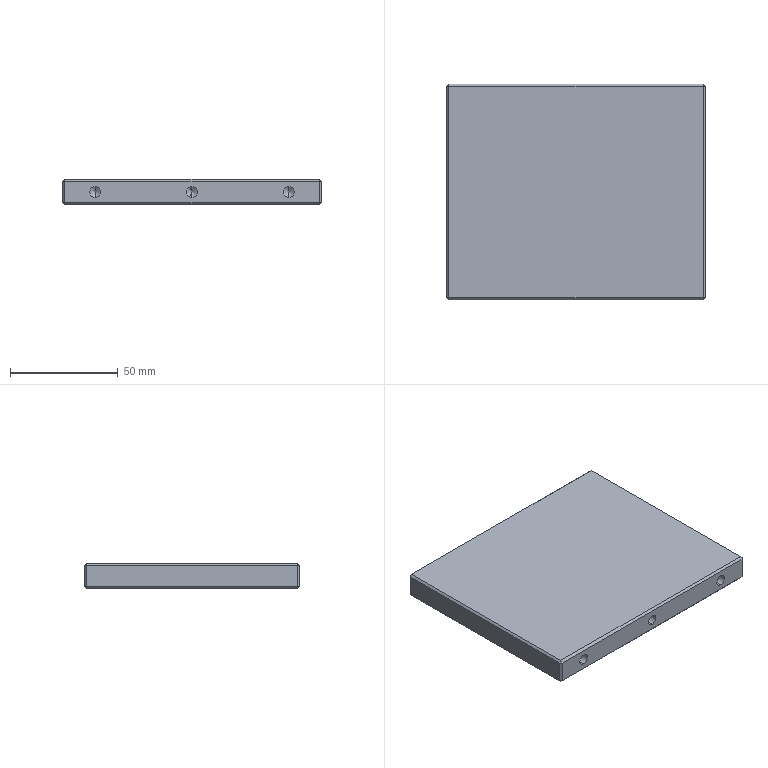Part | STEP file | 07-02 support plate | 1 solid | 49 faces | box 120 x 100 x 12 mm | volume 141828 mm3 | plane 27 | cylinder 12 | cone 10 | commonest cylinder face diameters 5 x6 4.2 x4 6 x2
STEP:
#1=CARTESIAN_POINT('',(0.,40.,3.));
#2=VERTEX_POINT('',#1);
#3=CARTESIAN_POINT('',(0.,40.,9.));
#4=VERTEX_POINT('',#3);
#5=CARTESIAN_POINT('',(0.,40.,6.));
#6=DIRECTION('',(0.,1.,0.));
#7=DIRECTION('',(0.,0.,1.));
#8=AXIS2_PLACEMENT_3D('',#5,#6,#7);
#9=CIRCLE('',#8,3.);
#10=EDGE_CURVE('',#2,#4,#9,.T.);
#11=ORIENTED_EDGE('',*,*,#10,.F.);
#12=CARTESIAN_POINT('',(0.,50.,3.));
#13=VERTEX_POINT('',#12);
#14=CARTESIAN_POINT('',(0.,40.,3.));
#15=DIRECTION('',(0.,1.,0.));
#16=VECTOR('',#15,1000.);
#17=LINE('',#14,#16);
#18=EDGE_CURVE('',#2,#13,#17,.T.);
#19=ORIENTED_EDGE('',*,*,#18,.T.);
#20=CARTESIAN_POINT('',(0.,50.,9.));
#21=VERTEX_POINT('',#20);
#22=CARTESIAN_POINT('',(0.,50.,6.));
#23=DIRECTION('',(0.,1.,0.));
#24=DIRECTION('',(0.,0.,1.));
#25=AXIS2_PLACEMENT_3D('',#22,#23,#24);
#26=CIRCLE('',#25,3.);
#27=EDGE_CURVE('',#13,#21,#26,.T.);
#28=ORIENTED_EDGE('',*,*,#27,.T.);
#29=CARTESIAN_POINT('',(0.,40.,9.));
#30=DIRECTION('',(0.,1.,0.));
#31=VECTOR('',#30,1000.);
#32=LINE('',#29,#31);
#33=EDGE_CURVE('',#4,#21,#32,.T.);
#34=ORIENTED_EDGE('',*,*,#33,.F.);
#35=EDGE_LOOP('',(#11,#19,#28,#34));
#36=FACE_OUTER_BOUND('',#35,.T.);
#37=CARTESIAN_POINT('',(0.,40.,6.));
#38=DIRECTION('',(0.,1.,0.));
#39=DIRECTION('',(0.,0.,1.));
#40=AXIS2_PLACEMENT_3D('',#37,#38,#39);
#41=CYLINDRICAL_SURFACE('',#40,3.);
#42=ADVANCED_FACE('',(#36),#41,.F.);
#43=CARTESIAN_POINT('',(-45.,36.,3.9));
#44=VERTEX_POINT('',#43);
#45=CARTESIAN_POINT('',(-45.,36.,8.1));
#46=VERTEX_POINT('',#45);
#47=CARTESIAN_POINT('',(-45.,36.,6.));
#48=DIRECTION('',(0.,1.,0.));
#49=DIRECTION('',(0.,0.,1.));
#50=AXIS2_PLACEMENT_3D('',#47,#48,#49);
#51=CIRCLE('',#50,2.1);
#52=EDGE_CURVE('',#44,#46,#51,.T.);
#53=ORIENTED_EDGE('',*,*,#52,.F.);
#54=CARTESIAN_POINT('',(-45.,50.,3.9));
#55=VERTEX_POINT('',#54);
#56=CARTESIAN_POINT('',(-45.,50.,3.9));
#57=DIRECTION('',(0.,1.,0.));
#58=VECTOR('',#57,1000.);
#59=LINE('',#56,#58);
#60=EDGE_CURVE('',#44,#55,#59,.T.);
#61=ORIENTED_EDGE('',*,*,#60,.T.);
#62=CARTESIAN_POINT('',(-45.,50.,8.1));
#63=VERTEX_POINT('',#62);
#64=CARTESIAN_POINT('',(-45.,50.,6.));
#65=DIRECTION('',(0.,1.,0.));
#66=DIRECTION('',(0.,0.,1.));
#67=AXIS2_PLACEMENT_3D('',#64,#65,#66);
#68=CIRCLE('',#67,2.1);
#69=EDGE_CURVE('',#55,#63,#68,.T.);
#70=ORIENTED_EDGE('',*,*,#69,.T.);
#71=CARTESIAN_POINT('',(-45.,50.,8.1));
#72=DIRECTION('',(0.,1.,0.));
#73=VECTOR('',#72,1000.);
#74=LINE('',#71,#73);
#75=EDGE_CURVE('',#46,#63,#74,.T.);
#76=ORIENTED_EDGE('',*,*,#75,.F.);
#77=EDGE_LOOP('',(#53,#61,#70,#76));
#78=FACE_OUTER_BOUND('',#77,.T.);
#79=CARTESIAN_POINT('',(-45.,50.,6.));
#80=DIRECTION('',(0.,1.,0.));
#81=DIRECTION('',(0.,0.,1.));
#82=AXIS2_PLACEMENT_3D('',#79,#80,#81);
#83=CYLINDRICAL_SURFACE('',#82,2.1);
#84=ADVANCED_FACE('',(#78),#83,.F.);
#85=CARTESIAN_POINT('',(-45.,34.738,6.));
#86=VERTEX_POINT('',#85);
#87=CARTESIAN_POINT('',(-45.,36.,8.1));
#88=DIRECTION('',(0.,0.515,0.8572));
#89=VECTOR('',#88,1000.);
#90=LINE('',#87,#89);
#91=EDGE_CURVE('',#86,#46,#90,.T.);
#92=ORIENTED_EDGE('',*,*,#91,.F.);
#93=CARTESIAN_POINT('',(-45.,36.,3.9));
#94=DIRECTION('',(0.,0.515,-0.8572));
#95=VECTOR('',#94,1000.);
#96=LINE('',#93,#95);
#97=EDGE_CURVE('',#86,#44,#96,.T.);
#98=ORIENTED_EDGE('',*,*,#97,.T.);
#99=ORIENTED_EDGE('',*,*,#52,.T.);
#100=EDGE_LOOP('',(#92,#98,#99));
#101=FACE_OUTER_BOUND('',#100,.T.);
#102=CARTESIAN_POINT('',(-45.,36.,6.));
#103=DIRECTION('',(0.,1.,0.));
#104=DIRECTION('',(0.,0.,1.));
#105=AXIS2_PLACEMENT_3D('',#102,#103,#104);
#106=CONICAL_SURFACE('',#105,2.1,1.03);
#107=ADVANCED_FACE('',(#101),#106,.F.);
#108=CARTESIAN_POINT('',(45.,36.,3.9));
#109=VERTEX_POINT('',#108);
#110=CARTESIAN_POINT('',(45.,36.,8.1));
#111=VERTEX_POINT('',#110);
#112=CARTESIAN_POINT('',(45.,36.,6.));
#113=DIRECTION('',(0.,1.,0.));
#114=DIRECTION('',(0.,0.,1.));
#115=AXIS2_PLACEMENT_3D('',#112,#113,#114);
#116=CIRCLE('',#115,2.1);
#117=EDGE_CURVE('',#109,#111,#116,.T.);
#118=ORIENTED_EDGE('',*,*,#117,.F.);
#119=CARTESIAN_POINT('',(45.,50.,3.9));
#120=VERTEX_POINT('',#119);
#121=CARTESIAN_POINT('',(45.,50.,3.9));
#122=DIRECTION('',(0.,1.,0.));
#123=VECTOR('',#122,1000.);
#124=LINE('',#121,#123);
#125=EDGE_CURVE('',#109,#120,#124,.T.);
#126=ORIENTED_EDGE('',*,*,#125,.T.);
#127=CARTESIAN_POINT('',(45.,50.,8.1));
#128=VERTEX_POINT('',#127);
#129=CARTESIAN_POINT('',(45.,50.,6.));
#130=DIRECTION('',(0.,1.,0.));
#131=DIRECTION('',(0.,0.,1.));
#132=AXIS2_PLACEMENT_3D('',#129,#130,#131);
#133=CIRCLE('',#132,2.1);
#134=EDGE_CURVE('',#120,#128,#133,.T.);
#135=ORIENTED_EDGE('',*,*,#134,.T.);
#136=CARTESIAN_POINT('',(45.,50.,8.1));
#137=DIRECTION('',(0.,1.,0.));
#138=VECTOR('',#137,1000.);
#139=LINE('',#136,#138);
#140=EDGE_CURVE('',#111,#128,#139,.T.);
#141=ORIENTED_EDGE('',*,*,#140,.F.);
#142=EDGE_LOOP('',(#118,#126,#135,#141));
#143=FACE_OUTER_BOUND('',#142,.T.);
#144=CARTESIAN_POINT('',(45.,50.,6.));
#145=DIRECTION('',(0.,1.,0.));
#146=DIRECTION('',(0.,0.,1.));
#147=AXIS2_PLACEMENT_3D('',#144,#145,#146);
#148=CYLINDRICAL_SURFACE('',#147,2.1);
#149=ADVANCED_FACE('',(#143),#148,.F.);
#150=CARTESIAN_POINT('',(45.,34.738,6.));
#151=VERTEX_POINT('',#150);
#152=CARTESIAN_POINT('',(45.,36.,8.1));
#153=DIRECTION('',(0.,0.515,0.8572));
#154=VECTOR('',#153,1000.);
#155=LINE('',#152,#154);
#156=EDGE_CURVE('',#151,#111,#155,.T.);
#157=ORIENTED_EDGE('',*,*,#156,.F.);
#158=CARTESIAN_POINT('',(45.,36.,3.9));
#159=DIRECTION('',(0.,0.515,-0.8572));
#160=VECTOR('',#159,1000.);
#161=LINE('',#158,#160);
#162=EDGE_CURVE('',#151,#109,#161,.T.);
#163=ORIENTED_EDGE('',*,*,#162,.T.);
#164=ORIENTED_EDGE('',*,*,#117,.T.);
#165=EDGE_LOOP('',(#157,#163,#164));
#166=FACE_OUTER_BOUND('',#165,.T.);
#167=CARTESIAN_POINT('',(45.,36.,6.));
#168=DIRECTION('',(0.,1.,0.));
#169=DIRECTION('',(0.,0.,1.));
#170=AXIS2_PLACEMENT_3D('',#167,#168,#169);
#171=CONICAL_SURFACE('',#170,2.1,1.03);
#172=ADVANCED_FACE('',(#166),#171,.F.);
#173=CARTESIAN_POINT('',(-45.,-33.,8.5));
#174=VERTEX_POINT('',#173);
#175=CARTESIAN_POINT('',(-45.,-33.,3.5));
#176=VERTEX_POINT('',#175);
#177=CARTESIAN_POINT('',(-45.,-33.,6.));
#178=DIRECTION('',(0.,-1.,0.));
#179=DIRECTION('',(0.,0.,-1.));
#180=AXIS2_PLACEMENT_3D('',#177,#178,#179);
#181=CIRCLE('',#180,2.5);
#182=EDGE_CURVE('',#174,#176,#181,.T.);
#183=ORIENTED_EDGE('',*,*,#182,.F.);
#184=CARTESIAN_POINT('',(-45.,-50.,8.5));
#185=VERTEX_POINT('',#184);
#186=CARTESIAN_POINT('',(-45.,-50.,8.5));
#187=DIRECTION('',(0.,-1.,0.));
#188=VECTOR('',#187,1000.);
#189=LINE('',#186,#188);
#190=EDGE_CURVE('',#174,#185,#189,.T.);
#191=ORIENTED_EDGE('',*,*,#190,.T.);
#192=CARTESIAN_POINT('',(-45.,-50.,3.5));
#193=VERTEX_POINT('',#192);
#194=CARTESIAN_POINT('',(-45.,-50.,6.));
#195=DIRECTION('',(0.,-1.,0.));
#196=DIRECTION('',(0.,0.,-1.));
#197=AXIS2_PLACEMENT_3D('',#194,#195,#196);
#198=CIRCLE('',#197,2.5);
#199=EDGE_CURVE('',#185,#193,#198,.T.);
#200=ORIENTED_EDGE('',*,*,#199,.T.);
#201=CARTESIAN_POINT('',(-45.,-50.,3.5));
#202=DIRECTION('',(0.,-1.,0.));
#203=VECTOR('',#202,1000.);
#204=LINE('',#201,#203);
#205=EDGE_CURVE('',#176,#193,#204,.T.);
#206=ORIENTED_EDGE('',*,*,#205,.F.);
#207=EDGE_LOOP('',(#183,#191,#200,#206));
#208=FACE_OUTER_BOUND('',#207,.T.);
#209=CARTESIAN_POINT('',(-45.,-50.,6.));
#210=DIRECTION('',(0.,-1.,0.));
#211=DIRECTION('',(0.,0.,-1.));
#212=AXIS2_PLACEMENT_3D('',#209,#210,#211);
#213=CYLINDRICAL_SURFACE('',#212,2.5);
#214=ADVANCED_FACE('',(#208),#213,.F.);
#215=CARTESIAN_POINT('',(-45.,-31.498,6.));
#216=VERTEX_POINT('',#215);
#217=CARTESIAN_POINT('',(-45.,-33.,3.5));
#218=DIRECTION('',(0.,-0.515,-0.8572));
#219=VECTOR('',#218,1000.);
#220=LINE('',#217,#219);
#221=EDGE_CURVE('',#216,#176,#220,.T.);
#222=ORIENTED_EDGE('',*,*,#221,.F.);
#223=CARTESIAN_POINT('',(-45.,-33.,8.5));
#224=DIRECTION('',(0.,-0.515,0.8572));
#225=VECTOR('',#224,1000.);
#226=LINE('',#223,#225);
#227=EDGE_CURVE('',#216,#174,#226,.T.);
#228=ORIENTED_EDGE('',*,*,#227,.T.);
#229=ORIENTED_EDGE('',*,*,#182,.T.);
#230=EDGE_LOOP('',(#222,#228,#229));
#231=FACE_OUTER_BOUND('',#230,.T.);
#232=CARTESIAN_POINT('',(-45.,-33.,6.));
#233=DIRECTION('',(0.,-1.,0.));
#234=DIRECTION('',(0.,0.,-1.));
#235=AXIS2_PLACEMENT_3D('',#232,#233,#234);
#236=CONICAL_SURFACE('',#235,2.5,1.03);
#237=ADVANCED_FACE('',(#231),#236,.F.);
#238=CARTESIAN_POINT('',(0.,-33.,8.5));
#239=VERTEX_POINT('',#238);
#240=CARTESIAN_POINT('',(0.,-33.,3.5));
#241=VERTEX_POINT('',#240);
#242=CARTESIAN_POINT('',(0.,-33.,6.));
#243=DIRECTION('',(0.,-1.,0.));
#244=DIRECTION('',(0.,0.,-1.));
#245=AXIS2_PLACEMENT_3D('',#242,#243,#244);
#246=CIRCLE('',#245,2.5);
#247=EDGE_CURVE('',#239,#241,#246,.T.);
#248=ORIENTED_EDGE('',*,*,#247,.F.);
#249=CARTESIAN_POINT('',(0.,-50.,8.5));
#250=VERTEX_POINT('',#249);
#251=CARTESIAN_POINT('',(0.,-50.,8.5));
#252=DIRECTION('',(0.,-1.,0.));
#253=VECTOR('',#252,1000.);
#254=LINE('',#251,#253);
#255=EDGE_CURVE('',#239,#250,#254,.T.);
#256=ORIENTED_EDGE('',*,*,#255,.T.);
#257=CARTESIAN_POINT('',(0.,-50.,3.5));
#258=VERTEX_POINT('',#257);
#259=CARTESIAN_POINT('',(0.,-50.,6.));
#260=DIRECTION('',(0.,-1.,0.));
#261=DIRECTION('',(0.,0.,-1.));
#262=AXIS2_PLACEMENT_3D('',#259,#260,#261);
#263=CIRCLE('',#262,2.5);
#264=EDGE_CURVE('',#250,#258,#263,.T.);
#265=ORIENTED_EDGE('',*,*,#264,.T.);
#266=CARTESIAN_POINT('',(0.,-50.,3.5));
#267=DIRECTION('',(0.,-1.,0.));
#268=VECTOR('',#267,1000.);
#269=LINE('',#266,#268);
#270=EDGE_CURVE('',#241,#258,#269,.T.);
#271=ORIENTED_EDGE('',*,*,#270,.F.);
#272=EDGE_LOOP('',(#248,#256,#265,#271));
#273=FACE_OUTER_BOUND('',#272,.T.);
#274=CARTESIAN_POINT('',(0.,-50.,6.));
#275=DIRECTION('',(0.,-1.,0.));
#276=DIRECTION('',(0.,0.,-1.));
#277=AXIS2_PLACEMENT_3D('',#274,#275,#276);
#278=CYLINDRICAL_SURFACE('',#277,2.5);
#279=ADVANCED_FACE('',(#273),#278,.F.);
#280=CARTESIAN_POINT('',(0.,-31.498,6.));
#281=VERTEX_POINT('',#280);
#282=CARTESIAN_POINT('',(0.,-33.,3.5));
#283=DIRECTION('',(0.,-0.515,-0.8572));
#284=VECTOR('',#283,1000.);
#285=LINE('',#282,#284);
#286=EDGE_CURVE('',#281,#241,#285,.T.);
#287=ORIENTED_EDGE('',*,*,#286,.F.);
#288=CARTESIAN_POINT('',(0.,-33.,8.5));
#289=DIRECTION('',(0.,-0.515,0.8572));
#290=VECTOR('',#289,1000.);
#291=LINE('',#288,#290);
#292=EDGE_CURVE('',#281,#239,#291,.T.);
#293=ORIENTED_EDGE('',*,*,#292,.T.);
#294=ORIENTED_EDGE('',*,*,#247,.T.);
#295=EDGE_LOOP('',(#287,#293,#294));
#296=FACE_OUTER_BOUND('',#295,.T.);
#297=CARTESIAN_POINT('',(0.,-33.,6.));
#298=DIRECTION('',(0.,-1.,0.));
#299=DIRECTION('',(0.,0.,-1.));
#300=AXIS2_PLACEMENT_3D('',#297,#298,#299);
#301=CONICAL_SURFACE('',#300,2.5,1.03);
#302=ADVANCED_FACE('',(#296),#301,.F.);
#303=CARTESIAN_POINT('',(45.,-33.,8.5));
#304=VERTEX_POINT('',#303);
#305=CARTESIAN_POINT('',(45.,-33.,3.5));
#306=VERTEX_POINT('',#305);
#307=CARTESIAN_POINT('',(45.,-33.,6.));
#308=DIRECTION('',(0.,-1.,0.));
#309=DIRECTION('',(0.,0.,-1.));
#310=AXIS2_PLACEMENT_3D('',#307,#308,#309);
#311=CIRCLE('',#310,2.5);
#312=EDGE_CURVE('',#304,#306,#311,.T.);
#313=ORIENTED_EDGE('',*,*,#312,.F.);
#314=CARTESIAN_POINT('',(45.,-50.,8.5));
#315=VERTEX_POINT('',#314);
#316=CARTESIAN_POINT('',(45.,-50.,8.5));
#317=DIRECTION('',(0.,-1.,0.));
#318=VECTOR('',#317,1000.);
#319=LINE('',#316,#318);
#320=EDGE_CURVE('',#304,#315,#319,.T.);
#321=ORIENTED_EDGE('',*,*,#320,.T.);
#322=CARTESIAN_POINT('',(45.,-50.,3.5));
#323=VERTEX_POINT('',#322);
#324=CARTESIAN_POINT('',(45.,-50.,6.));
#325=DIRECTION('',(0.,-1.,0.));
#326=DIRECTION('',(0.,0.,-1.));
#327=AXIS2_PLACEMENT_3D('',#324,#325,#326);
#328=CIRCLE('',#327,2.5);
#329=EDGE_CURVE('',#315,#323,#328,.T.);
#330=ORIENTED_EDGE('',*,*,#329,.T.);
#331=CARTESIAN_POINT('',(45.,-50.,3.5));
#332=DIRECTION('',(0.,-1.,0.));
#333=VECTOR('',#332,1000.);
#334=LINE('',#331,#333);
#335=EDGE_CURVE('',#306,#323,#334,.T.);
#336=ORIENTED_EDGE('',*,*,#335,.F.);
#337=EDGE_LOOP('',(#313,#321,#330,#336));
#338=FACE_OUTER_BOUND('',#337,.T.);
#339=CARTESIAN_POINT('',(45.,-50.,6.));
#340=DIRECTION('',(0.,-1.,0.));
#341=DIRECTION('',(0.,0.,-1.));
#342=AXIS2_PLACEMENT_3D('',#339,#340,#341);
#343=CYLINDRICAL_SURFACE('',#342,2.5);
#344=ADVANCED_FACE('',(#338),#343,.F.);
#345=CARTESIAN_POINT('',(45.,-31.498,6.));
#346=VERTEX_POINT('',#345);
#347=CARTESIAN_POINT('',(45.,-33.,3.5));
#348=DIRECTION('',(0.,-0.515,-0.8572));
#349=VECTOR('',#348,1000.);
#350=LINE('',#347,#349);
#351=EDGE_CURVE('',#346,#306,#350,.T.);
#352=ORIENTED_EDGE('',*,*,#351,.F.);
#353=CARTESIAN_POINT('',(45.,-33.,8.5));
#354=DIRECTION('',(0.,-0.515,0.8572));
#355=VECTOR('',#354,1000.);
#356=LINE('',#353,#355);
#357=EDGE_CURVE('',#346,#304,#356,.T.);
#358=ORIENTED_EDGE('',*,*,#357,.T.);
#359=ORIENTED_EDGE('',*,*,#312,.T.);
#360=EDGE_LOOP('',(#352,#358,#359));
#361=FACE_OUTER_BOUND('',#360,.T.);
#362=CARTESIAN_POINT('',(45.,-33.,6.));
#363=DIRECTION('',(0.,-1.,0.));
#364=DIRECTION('',(0.,0.,-1.));
#365=AXIS2_PLACEMENT_3D('',#362,#363,#364);
#366=CONICAL_SURFACE('',#365,2.5,1.03);
#367=ADVANCED_FACE('',(#361),#366,.F.);
#368=CARTESIAN_POINT('',(60.,-49.,11.));
#369=VERTEX_POINT('',#368);
#370=CARTESIAN_POINT('',(60.,-49.,1.));
#371=VERTEX_POINT('',#370);
#372=CARTESIAN_POINT('',(60.,-49.,12.));
#373=DIRECTION('',(0.,0.,-1.));
#374=VECTOR('',#373,1000.);
#375=LINE('',#372,#374);
#376=EDGE_CURVE('',#369,#371,#375,.T.);
#377=ORIENTED_EDGE('',*,*,#376,.T.);
#378=CARTESIAN_POINT('',(60.,49.,1.));
#379=VERTEX_POINT('',#378);
#380=CARTESIAN_POINT('',(60.,50.,1.));
#381=DIRECTION('',(0.,1.,0.));
#382=VECTOR('',#381,1000.);
#383=LINE('',#380,#382);
#384=EDGE_CURVE('',#371,#379,#383,.T.);
#385=ORIENTED_EDGE('',*,*,#384,.T.);
#386=CARTESIAN_POINT('',(60.,49.,11.));
#387=VERTEX_POINT('',#386);
#388=CARTESIAN_POINT('',(60.,49.,12.));
#389=DIRECTION('',(0.,0.,1.));
#390=VECTOR('',#389,1000.);
#391=LINE('',#388,#390);
#392=EDGE_CURVE('',#379,#387,#391,.T.);
#393=ORIENTED_EDGE('',*,*,#392,.T.);
#394=CARTESIAN_POINT('',(60.,-50.,11.));
#395=DIRECTION('',(0.,-1.,0.));
#396=VECTOR('',#395,1000.);
#397=LINE('',#394,#396);
#398=EDGE_CURVE('',#387,#369,#397,.T.);
#399=ORIENTED_EDGE('',*,*,#398,.T.);
#400=EDGE_LOOP('',(#377,#385,#393,#399));
#401=FACE_OUTER_BOUND('',#400,.T.);
#402=CARTESIAN_POINT('',(60.,50.,12.));
#403=DIRECTION('',(-1.,0.,0.));
#404=DIRECTION('',(0.,-1.,0.));
#405=AXIS2_PLACEMENT_3D('',#402,#403,#404);
#406=PLANE('',#405);
#407=ADVANCED_FACE('',(#401),#406,.F.);
#408=CARTESIAN_POINT('',(59.,50.,11.));
#409=VERTEX_POINT('',#408);
#410=CARTESIAN_POINT('',(59.,50.,1.));
#411=VERTEX_POINT('',#410);
#412=CARTESIAN_POINT('',(59.,50.,12.));
#413=DIRECTION('',(0.,0.,-1.));
#414=VECTOR('',#413,1000.);
#415=LINE('',#412,#414);
#416=EDGE_CURVE('',#409,#411,#415,.T.);
#417=ORIENTED_EDGE('',*,*,#416,.T.);
#418=CARTESIAN_POINT('',(-59.,50.,1.));
#419=VERTEX_POINT('',#418);
#420=CARTESIAN_POINT('',(-60.,50.,1.));
#421=DIRECTION('',(-1.,0.,0.));
#422=VECTOR('',#421,1000.);
#423=LINE('',#420,#422);
#424=EDGE_CURVE('',#411,#419,#423,.T.);
#425=ORIENTED_EDGE('',*,*,#424,.T.);
#426=CARTESIAN_POINT('',(-59.,50.,11.));
#427=VERTEX_POINT('',#426);
#428=CARTESIAN_POINT('',(-59.,50.,12.));
#429=DIRECTION('',(0.,0.,1.));
#430=VECTOR('',#429,1000.);
#431=LINE('',#428,#430);
#432=EDGE_CURVE('',#419,#427,#431,.T.);
#433=ORIENTED_EDGE('',*,*,#432,.T.);
#434=CARTESIAN_POINT('',(60.,50.,11.));
#435=DIRECTION('',(1.,0.,0.));
#436=VECTOR('',#435,1000.);
#437=LINE('',#434,#436);
#438=EDGE_CURVE('',#427,#409,#437,.T.);
#439=ORIENTED_EDGE('',*,*,#438,.T.);
#440=EDGE_LOOP('',(#417,#425,#433,#439));
#441=FACE_OUTER_BOUND('',#440,.T.);
#442=CARTESIAN_POINT('',(0.,50.,6.));
#443=DIRECTION('',(0.,1.,0.));
#444=DIRECTION('',(0.,0.,1.));
#445=AXIS2_PLACEMENT_3D('',#442,#443,#444);
#446=CIRCLE('',#445,3.);
#447=EDGE_CURVE('',#21,#13,#446,.T.);
#448=ORIENTED_EDGE('',*,*,#447,.F.);
#449=ORIENTED_EDGE('',*,*,#27,.F.);
#450=EDGE_LOOP('',(#448,#449));
#451=FACE_BOUND('',#450,.T.);
#452=CARTESIAN_POINT('',(-45.,50.,6.));
#453=DIRECTION('',(0.,1.,0.));
#454=DIRECTION('',(0.,0.,1.));
#455=AXIS2_PLACEMENT_3D('',#452,#453,#454);
#456=CIRCLE('',#455,2.1);
#457=EDGE_CURVE('',#63,#55,#456,.T.);
#458=ORIENTED_EDGE('',*,*,#457,.F.);
#459=ORIENTED_EDGE('',*,*,#69,.F.);
#460=EDGE_LOOP('',(#458,#459));
#461=FACE_BOUND('',#460,.T.);
#462=CARTESIAN_POINT('',(45.,50.,6.));
#463=DIRECTION('',(0.,1.,0.));
#464=DIRECTION('',(0.,0.,1.));
#465=AXIS2_PLACEMENT_3D('',#462,#463,#464);
#466=CIRCLE('',#465,2.1);
#467=EDGE_CURVE('',#128,#120,#466,.T.);
#468=ORIENTED_EDGE('',*,*,#467,.F.);
#469=ORIENTED_EDGE('',*,*,#134,.F.);
#470=EDGE_LOOP('',(#468,#469));
#471=FACE_BOUND('',#470,.T.);
#472=CARTESIAN_POINT('',(-60.,50.,12.));
#473=DIRECTION('',(0.,-1.,0.));
#474=DIRECTION('',(0.,0.,-1.));
#475=AXIS2_PLACEMENT_3D('',#472,#473,#474);
#476=PLANE('',#475);
#477=ADVANCED_FACE('',(#441,#451,#461,#471),#476,.F.);
#478=CARTESIAN_POINT('',(-60.,49.,11.));
#479=VERTEX_POINT('',#478);
#480=CARTESIAN_POINT('',(-60.,49.,1.));
#481=VERTEX_POINT('',#480);
#482=CARTESIAN_POINT('',(-60.,49.,12.));
#483=DIRECTION('',(0.,0.,-1.));
#484=VECTOR('',#483,1000.);
#485=LINE('',#482,#484);
#486=EDGE_CURVE('',#479,#481,#485,.T.);
#487=ORIENTED_EDGE('',*,*,#486,.T.);
#488=CARTESIAN_POINT('',(-60.,-49.,1.));
#489=VERTEX_POINT('',#488);
#490=CARTESIAN_POINT('',(-60.,50.,1.));
#491=DIRECTION('',(0.,-1.,0.));
#492=VECTOR('',#491,1000.);
#493=LINE('',#490,#492);
#494=EDGE_CURVE('',#481,#489,#493,.T.);
#495=ORIENTED_EDGE('',*,*,#494,.T.);
#496=CARTESIAN_POINT('',(-60.,-49.,11.));
#497=VERTEX_POINT('',#496);
#498=CARTESIAN_POINT('',(-60.,-49.,12.));
#499=DIRECTION('',(0.,0.,1.));
#500=VECTOR('',#499,1000.);
#501=LINE('',#498,#500);
#502=EDGE_CURVE('',#489,#497,#501,.T.);
#503=ORIENTED_EDGE('',*,*,#502,.T.);
#504=CARTESIAN_POINT('',(-60.,50.,11.));
#505=DIRECTION('',(0.,1.,0.));
#506=VECTOR('',#505,1000.);
#507=LINE('',#504,#506);
#508=EDGE_CURVE('',#497,#479,#507,.T.);
#509=ORIENTED_EDGE('',*,*,#508,.T.);
#510=EDGE_LOOP('',(#487,#495,#503,#509));
#511=FACE_OUTER_BOUND('',#510,.T.);
#512=CARTESIAN_POINT('',(-60.,50.,12.));
#513=DIRECTION('',(1.,0.,0.));
#514=DIRECTION('',(0.,1.,0.));
#515=AXIS2_PLACEMENT_3D('',#512,#513,#514);
#516=PLANE('',#515);
#517=ADVANCED_FACE('',(#511),#516,.F.);
#518=CARTESIAN_POINT('',(59.,-50.,11.));
#519=VERTEX_POINT('',#518);
#520=CARTESIAN_POINT('',(-59.,-50.,11.));
#521=VERTEX_POINT('',#520);
#522=CARTESIAN_POINT('',(-60.,-50.,11.));
#523=DIRECTION('',(-1.,0.,0.));
#524=VECTOR('',#523,1000.);
#525=LINE('',#522,#524);
#526=EDGE_CURVE('',#519,#521,#525,.T.);
#527=ORIENTED_EDGE('',*,*,#526,.T.);
#528=CARTESIAN_POINT('',(-59.,-50.,1.));
#529=VERTEX_POINT('',#528);
#530=CARTESIAN_POINT('',(-59.,-50.,12.));
#531=DIRECTION('',(0.,0.,-1.));
#532=VECTOR('',#531,1000.);
#533=LINE('',#530,#532);
#534=EDGE_CURVE('',#521,#529,#533,.T.);
#535=ORIENTED_EDGE('',*,*,#534,.T.);
#536=CARTESIAN_POINT('',(59.,-50.,1.));
#537=VERTEX_POINT('',#536);
#538=CARTESIAN_POINT('',(-60.,-50.,1.));
#539=DIRECTION('',(1.,0.,0.));
#540=VECTOR('',#539,1000.);
#541=LINE('',#538,#540);
#542=EDGE_CURVE('',#529,#537,#541,.T.);
#543=ORIENTED_EDGE('',*,*,#542,.T.);
#544=CARTESIAN_POINT('',(59.,-50.,12.));
#545=DIRECTION('',(0.,0.,1.));
#546=VECTOR('',#545,1000.);
#547=LINE('',#544,#546);
#548=EDGE_CURVE('',#537,#519,#547,.T.);
#549=ORIENTED_EDGE('',*,*,#548,.T.);
#550=EDGE_LOOP('',(#527,#535,#543,#549));
#551=FACE_OUTER_BOUND('',#550,.T.);
#552=CARTESIAN_POINT('',(-45.,-50.,6.));
#553=DIRECTION('',(0.,-1.,0.));
#554=DIRECTION('',(0.,0.,-1.));
#555=AXIS2_PLACEMENT_3D('',#552,#553,#554);
#556=CIRCLE('',#555,2.5);
#557=EDGE_CURVE('',#193,#185,#556,.T.);
#558=ORIENTED_EDGE('',*,*,#557,.F.);
#559=ORIENTED_EDGE('',*,*,#199,.F.);
#560=EDGE_LOOP('',(#558,#559));
#561=FACE_BOUND('',#560,.T.);
#562=CARTESIAN_POINT('',(0.,-50.,6.));
#563=DIRECTION('',(0.,-1.,0.));
#564=DIRECTION('',(0.,0.,-1.));
#565=AXIS2_PLACEMENT_3D('',#562,#563,#564);
#566=CIRCLE('',#565,2.5);
#567=EDGE_CURVE('',#258,#250,#566,.T.);
#568=ORIENTED_EDGE('',*,*,#567,.F.);
#569=ORIENTED_EDGE('',*,*,#264,.F.);
#570=EDGE_LOOP('',(#568,#569));
#571=FACE_BOUND('',#570,.T.);
#572=CARTESIAN_POINT('',(45.,-50.,6.));
#573=DIRECTION('',(0.,-1.,0.));
#574=DIRECTION('',(0.,0.,-1.));
#575=AXIS2_PLACEMENT_3D('',#572,#573,#574);
#576=CIRCLE('',#575,2.5);
#577=EDGE_CURVE('',#323,#315,#576,.T.);
#578=ORIENTED_EDGE('',*,*,#577,.F.);
#579=ORIENTED_EDGE('',*,*,#329,.F.);
#580=EDGE_LOOP('',(#578,#579));
#581=FACE_BOUND('',#580,.T.);
#582=CARTESIAN_POINT('',(-60.,-50.,12.));
#583=DIRECTION('',(0.,1.,0.));
#584=DIRECTION('',(0.,0.,1.));
#585=AXIS2_PLACEMENT_3D('',#582,#583,#584);
#586=PLANE('',#585);
#587=ADVANCED_FACE('',(#551,#561,#571,#581),#586,.F.);
#588=CARTESIAN_POINT('',(-59.,49.,12.));
#589=VERTEX_POINT('',#588);
#590=CARTESIAN_POINT('',(-59.,-49.,12.));
#591=VERTEX_POINT('',#590);
#592=CARTESIAN_POINT('',(-59.,-50.,12.));
#593=DIRECTION('',(0.,-1.,0.));
#594=VECTOR('',#593,1000.);
#595=LINE('',#592,#594);
#596=EDGE_CURVE('',#589,#591,#595,.T.);
#597=ORIENTED_EDGE('',*,*,#596,.T.);
#598=CARTESIAN_POINT('',(59.,-49.,12.));
#599=VERTEX_POINT('',#598);
#600=CARTESIAN_POINT('',(60.,-49.,12.));
#601=DIRECTION('',(1.,0.,0.));
#602=VECTOR('',#601,1000.);
#603=LINE('',#600,#602);
#604=EDGE_CURVE('',#591,#599,#603,.T.);
#605=ORIENTED_EDGE('',*,*,#604,.T.);
#606=CARTESIAN_POINT('',(59.,49.,12.));
#607=VERTEX_POINT('',#606);
#608=CARTESIAN_POINT('',(59.,50.,12.));
#609=DIRECTION('',(0.,1.,0.));
#610=VECTOR('',#609,1000.);
#611=LINE('',#608,#610);
#612=EDGE_CURVE('',#599,#607,#611,.T.);
#613=ORIENTED_EDGE('',*,*,#612,.T.);
#614=CARTESIAN_POINT('',(-60.,49.,12.));
#615=DIRECTION('',(-1.,0.,0.));
#616=VECTOR('',#615,1000.);
#617=LINE('',#614,#616);
#618=EDGE_CURVE('',#607,#589,#617,.T.);
#619=ORIENTED_EDGE('',*,*,#618,.T.);
#620=EDGE_LOOP('',(#597,#605,#613,#619));
#621=FACE_OUTER_BOUND('',#620,.T.);
#622=CARTESIAN_POINT('',(60.,-50.,12.));
#623=DIRECTION('',(0.,0.,1.));
#624=DIRECTION('',(1.,0.,0.));
#625=AXIS2_PLACEMENT_3D('',#622,#623,#624);
#626=PLANE('',#625);
#627=ADVANCED_FACE('',(#621),#626,.T.);
#628=CARTESIAN_POINT('',(-59.,-49.,0.));
#629=VERTEX_POINT('',#628);
#630=CARTESIAN_POINT('',(-59.,49.,0.));
#631=VERTEX_POINT('',#630);
#632=CARTESIAN_POINT('',(-59.,-50.,0.));
#633=DIRECTION('',(0.,1.,0.));
#634=VECTOR('',#633,1000.);
#635=LINE('',#632,#634);
#636=EDGE_CURVE('',#629,#631,#635,.T.);
#637=ORIENTED_EDGE('',*,*,#636,.T.);
#638=CARTESIAN_POINT('',(59.,49.,0.));
#639=VERTEX_POINT('',#638);
#640=CARTESIAN_POINT('',(60.,49.,0.));
#641=DIRECTION('',(1.,0.,0.));
#642=VECTOR('',#641,1000.);
#643=LINE('',#640,#642);
#644=EDGE_CURVE('',#631,#639,#643,.T.);
#645=ORIENTED_EDGE('',*,*,#644,.T.);
#646=CARTESIAN_POINT('',(59.,-49.,0.));
#647=VERTEX_POINT('',#646);
#648=CARTESIAN_POINT('',(59.,-50.,0.));
#649=DIRECTION('',(0.,-1.,0.));
#650=VECTOR('',#649,1000.);
#651=LINE('',#648,#650);
#652=EDGE_CURVE('',#639,#647,#651,.T.);
#653=ORIENTED_EDGE('',*,*,#652,.T.);
#654=CARTESIAN_POINT('',(60.,-49.,0.));
#655=DIRECTION('',(-1.,0.,0.));
#656=VECTOR('',#655,1000.);
#657=LINE('',#654,#656);
#658=EDGE_CURVE('',#647,#629,#657,.T.);
#659=ORIENTED_EDGE('',*,*,#658,.T.);
#660=EDGE_LOOP('',(#637,#645,#653,#659));
#661=FACE_OUTER_BOUND('',#660,.T.);
#662=CARTESIAN_POINT('',(60.,-50.,0.));
#663=DIRECTION('',(0.,0.,1.));
#664=DIRECTION('',(1.,0.,0.));
#665=AXIS2_PLACEMENT_3D('',#662,#663,#664);
#666=PLANE('',#665);
#667=ADVANCED_FACE('',(#661),#666,.F.);
#668=ORIENTED_EDGE('',*,*,#357,.F.);
#669=ORIENTED_EDGE('',*,*,#351,.T.);
#670=CARTESIAN_POINT('',(45.,-33.,6.));
#671=DIRECTION('',(0.,-1.,0.));
#672=DIRECTION('',(0.,0.,-1.));
#673=AXIS2_PLACEMENT_3D('',#670,#671,#672);
#674=CIRCLE('',#673,2.5);
#675=EDGE_CURVE('',#306,#304,#674,.T.);
#676=ORIENTED_EDGE('',*,*,#675,.T.);
#677=EDGE_LOOP('',(#668,#669,#676));
#678=FACE_OUTER_BOUND('',#677,.T.);
#679=CARTESIAN_POINT('',(45.,-33.,6.));
#680=DIRECTION('',(0.,-1.,0.));
#681=DIRECTION('',(0.,0.,-1.));
#682=AXIS2_PLACEMENT_3D('',#679,#680,#681);
#683=CONICAL_SURFACE('',#682,2.5,1.03);
#684=ADVANCED_FACE('',(#678),#683,.F.);
#685=ORIENTED_EDGE('',*,*,#320,.F.);
#686=ORIENTED_EDGE('',*,*,#675,.F.);
#687=ORIENTED_EDGE('',*,*,#335,.T.);
#688=ORIENTED_EDGE('',*,*,#577,.T.);
#689=EDGE_LOOP('',(#685,#686,#687,#688));
#690=FACE_OUTER_BOUND('',#689,.T.);
#691=CARTESIAN_POINT('',(45.,-50.,6.));
#692=DIRECTION('',(0.,-1.,0.));
#693=DIRECTION('',(0.,0.,-1.));
#694=AXIS2_PLACEMENT_3D('',#691,#692,#693);
#695=CYLINDRICAL_SURFACE('',#694,2.5);
#696=ADVANCED_FACE('',(#690),#695,.F.);
#697=ORIENTED_EDGE('',*,*,#292,.F.);
#698=ORIENTED_EDGE('',*,*,#286,.T.);
#699=CARTESIAN_POINT('',(0.,-33.,6.));
#700=DIRECTION('',(0.,-1.,0.));
#701=DIRECTION('',(0.,0.,-1.));
#702=AXIS2_PLACEMENT_3D('',#699,#700,#701);
#703=CIRCLE('',#702,2.5);
#704=EDGE_CURVE('',#241,#239,#703,.T.);
#705=ORIENTED_EDGE('',*,*,#704,.T.);
#706=EDGE_LOOP('',(#697,#698,#705));
#707=FACE_OUTER_BOUND('',#706,.T.);
#708=CARTESIAN_POINT('',(0.,-33.,6.));
#709=DIRECTION('',(0.,-1.,0.));
#710=DIRECTION('',(0.,0.,-1.));
#711=AXIS2_PLACEMENT_3D('',#708,#709,#710);
#712=CONICAL_SURFACE('',#711,2.5,1.03);
#713=ADVANCED_FACE('',(#707),#712,.F.);
#714=ORIENTED_EDGE('',*,*,#255,.F.);
#715=ORIENTED_EDGE('',*,*,#704,.F.);
#716=ORIENTED_EDGE('',*,*,#270,.T.);
#717=ORIENTED_EDGE('',*,*,#567,.T.);
#718=EDGE_LOOP('',(#714,#715,#716,#717));
#719=FACE_OUTER_BOUND('',#718,.T.);
#720=CARTESIAN_POINT('',(0.,-50.,6.));
#721=DIRECTION('',(0.,-1.,0.));
#722=DIRECTION('',(0.,0.,-1.));
#723=AXIS2_PLACEMENT_3D('',#720,#721,#722);
#724=CYLINDRICAL_SURFACE('',#723,2.5);
#725=ADVANCED_FACE('',(#719),#724,.F.);
#726=ORIENTED_EDGE('',*,*,#227,.F.);
#727=ORIENTED_EDGE('',*,*,#221,.T.);
#728=CARTESIAN_POINT('',(-45.,-33.,6.));
#729=DIRECTION('',(0.,-1.,0.));
#730=DIRECTION('',(0.,0.,-1.));
#731=AXIS2_PLACEMENT_3D('',#728,#729,#730);
#732=CIRCLE('',#731,2.5);
#733=EDGE_CURVE('',#176,#174,#732,.T.);
#734=ORIENTED_EDGE('',*,*,#733,.T.);
#735=EDGE_LOOP('',(#726,#727,#734));
#736=FACE_OUTER_BOUND('',#735,.T.);
#737=CARTESIAN_POINT('',(-45.,-33.,6.));
#738=DIRECTION('',(0.,-1.,0.));
#739=DIRECTION('',(0.,0.,-1.));
#740=AXIS2_PLACEMENT_3D('',#737,#738,#739);
#741=CONICAL_SURFACE('',#740,2.5,1.03);
#742=ADVANCED_FACE('',(#736),#741,.F.);
#743=ORIENTED_EDGE('',*,*,#190,.F.);
#744=ORIENTED_EDGE('',*,*,#733,.F.);
#745=ORIENTED_EDGE('',*,*,#205,.T.);
#746=ORIENTED_EDGE('',*,*,#557,.T.);
#747=EDGE_LOOP('',(#743,#744,#745,#746));
#748=FACE_OUTER_BOUND('',#747,.T.);
#749=CARTESIAN_POINT('',(-45.,-50.,6.));
#750=DIRECTION('',(0.,-1.,0.));
#751=DIRECTION('',(0.,0.,-1.));
#752=AXIS2_PLACEMENT_3D('',#749,#750,#751);
#753=CYLINDRICAL_SURFACE('',#752,2.5);
#754=ADVANCED_FACE('',(#748),#753,.F.);
#755=ORIENTED_EDGE('',*,*,#162,.F.);
#756=ORIENTED_EDGE('',*,*,#156,.T.);
#757=CARTESIAN_POINT('',(45.,36.,6.));
#758=DIRECTION('',(0.,1.,0.));
#759=DIRECTION('',(0.,0.,1.));
#760=AXIS2_PLACEMENT_3D('',#757,#758,#759);
#761=CIRCLE('',#760,2.1);
#762=EDGE_CURVE('',#111,#109,#761,.T.);
#763=ORIENTED_EDGE('',*,*,#762,.T.);
#764=EDGE_LOOP('',(#755,#756,#763));
#765=FACE_OUTER_BOUND('',#764,.T.);
#766=CARTESIAN_POINT('',(45.,36.,6.));
#767=DIRECTION('',(0.,1.,0.));
#768=DIRECTION('',(0.,0.,1.));
#769=AXIS2_PLACEMENT_3D('',#766,#767,#768);
#770=CONICAL_SURFACE('',#769,2.1,1.03);
#771=ADVANCED_FACE('',(#765),#770,.F.);
#772=ORIENTED_EDGE('',*,*,#125,.F.);
#773=ORIENTED_EDGE('',*,*,#762,.F.);
#774=ORIENTED_EDGE('',*,*,#140,.T.);
#775=ORIENTED_EDGE('',*,*,#467,.T.);
#776=EDGE_LOOP('',(#772,#773,#774,#775));
#777=FACE_OUTER_BOUND('',#776,.T.);
#778=CARTESIAN_POINT('',(45.,50.,6.));
#779=DIRECTION('',(0.,1.,0.));
#780=DIRECTION('',(0.,0.,1.));
#781=AXIS2_PLACEMENT_3D('',#778,#779,#780);
#782=CYLINDRICAL_SURFACE('',#781,2.1);
#783=ADVANCED_FACE('',(#777),#782,.F.);
#784=ORIENTED_EDGE('',*,*,#97,.F.);
#785=ORIENTED_EDGE('',*,*,#91,.T.);
#786=CARTESIAN_POINT('',(-45.,36.,6.));
#787=DIRECTION('',(0.,1.,0.));
#788=DIRECTION('',(0.,0.,1.));
#789=AXIS2_PLACEMENT_3D('',#786,#787,#788);
#790=CIRCLE('',#789,2.1);
#791=EDGE_CURVE('',#46,#44,#790,.T.);
#792=ORIENTED_EDGE('',*,*,#791,.T.);
#793=EDGE_LOOP('',(#784,#785,#792));
#794=FACE_OUTER_BOUND('',#793,.T.);
#795=CARTESIAN_POINT('',(-45.,36.,6.));
#796=DIRECTION('',(0.,1.,0.));
#797=DIRECTION('',(0.,0.,1.));
#798=AXIS2_PLACEMENT_3D('',#795,#796,#797);
#799=CONICAL_SURFACE('',#798,2.1,1.03);
#800=ADVANCED_FACE('',(#794),#799,.F.);
#801=ORIENTED_EDGE('',*,*,#60,.F.);
#802=ORIENTED_EDGE('',*,*,#791,.F.);
#803=ORIENTED_EDGE('',*,*,#75,.T.);
#804=ORIENTED_EDGE('',*,*,#457,.T.);
#805=EDGE_LOOP('',(#801,#802,#803,#804));
#806=FACE_OUTER_BOUND('',#805,.T.);
#807=CARTESIAN_POINT('',(-45.,50.,6.));
#808=DIRECTION('',(0.,1.,0.));
#809=DIRECTION('',(0.,0.,1.));
#810=AXIS2_PLACEMENT_3D('',#807,#808,#809);
#811=CYLINDRICAL_SURFACE('',#810,2.1);
#812=ADVANCED_FACE('',(#806),#811,.F.);
#813=ORIENTED_EDGE('',*,*,#18,.F.);
#814=CARTESIAN_POINT('',(0.,40.,6.));
#815=DIRECTION('',(0.,1.,0.));
#816=DIRECTION('',(0.,0.,1.));
#817=AXIS2_PLACEMENT_3D('',#814,#815,#816);
#818=CIRCLE('',#817,3.);
#819=EDGE_CURVE('',#4,#2,#818,.T.);
#820=ORIENTED_EDGE('',*,*,#819,.F.);
#821=ORIENTED_EDGE('',*,*,#33,.T.);
#822=ORIENTED_EDGE('',*,*,#447,.T.);
#823=EDGE_LOOP('',(#813,#820,#821,#822));
#824=FACE_OUTER_BOUND('',#823,.T.);
#825=CARTESIAN_POINT('',(0.,40.,6.));
#826=DIRECTION('',(0.,1.,0.));
#827=DIRECTION('',(0.,0.,1.));
#828=AXIS2_PLACEMENT_3D('',#825,#826,#827);
#829=CYLINDRICAL_SURFACE('',#828,3.);
#830=ADVANCED_FACE('',(#824),#829,.F.);
#831=ORIENTED_EDGE('',*,*,#819,.T.);
#832=ORIENTED_EDGE('',*,*,#10,.T.);
#833=EDGE_LOOP('',(#831,#832));
#834=FACE_OUTER_BOUND('',#833,.T.);
#835=CARTESIAN_POINT('',(0.,40.,6.));
#836=DIRECTION('',(0.,1.,0.));
#837=DIRECTION('',(0.,0.,1.));
#838=AXIS2_PLACEMENT_3D('',#835,#836,#837);
#839=PLANE('',#838);
#840=ADVANCED_FACE('',(#834),#839,.T.);
#841=CARTESIAN_POINT('',(59.,-49.,12.));
#842=DIRECTION('',(0.,-0.7071,-0.7071));
#843=VECTOR('',#842,1000.);
#844=LINE('',#841,#843);
#845=EDGE_CURVE('',#599,#519,#844,.T.);
#846=ORIENTED_EDGE('',*,*,#845,.F.);
#847=ORIENTED_EDGE('',*,*,#604,.F.);
#848=CARTESIAN_POINT('',(-59.,-50.,11.));
#849=DIRECTION('',(0.,0.7071,0.7071));
#850=VECTOR('',#849,1000.);
#851=LINE('',#848,#850);
#852=EDGE_CURVE('',#521,#591,#851,.T.);
#853=ORIENTED_EDGE('',*,*,#852,.F.);
#854=ORIENTED_EDGE('',*,*,#526,.F.);
#855=EDGE_LOOP('',(#846,#847,#853,#854));
#856=FACE_OUTER_BOUND('',#855,.T.);
#857=CARTESIAN_POINT('',(60.,-49.,12.));
#858=DIRECTION('',(0.,-0.7071,0.7071));
#859=DIRECTION('',(0.,-0.7071,-0.7071));
#860=AXIS2_PLACEMENT_3D('',#857,#858,#859);
#861=PLANE('',#860);
#862=ADVANCED_FACE('',(#856),#861,.T.);
#863=CARTESIAN_POINT('',(59.,-49.,12.));
#864=DIRECTION('',(0.7071,0.,-0.7071));
#865=VECTOR('',#864,1000.);
#866=LINE('',#863,#865);
#867=EDGE_CURVE('',#599,#369,#866,.T.);
#868=ORIENTED_EDGE('',*,*,#867,.F.);
#869=ORIENTED_EDGE('',*,*,#845,.T.);
#870=CARTESIAN_POINT('',(59.5,-49.5,11.));
#871=DIRECTION('',(-0.7071,-0.7071,0.));
#872=VECTOR('',#871,1000.);
#873=LINE('',#870,#872);
#874=EDGE_CURVE('',#369,#519,#873,.T.);
#875=ORIENTED_EDGE('',*,*,#874,.F.);
#876=EDGE_LOOP('',(#868,#869,#875));
#877=FACE_OUTER_BOUND('',#876,.T.);
#878=CARTESIAN_POINT('',(59.,-49.,12.));
#879=DIRECTION('',(0.5774,-0.5774,0.5774));
#880=DIRECTION('',(0.7071,0.7071,0.));
#881=AXIS2_PLACEMENT_3D('',#878,#879,#880);
#882=PLANE('',#881);
#883=ADVANCED_FACE('',(#877),#882,.T.);
#884=CARTESIAN_POINT('',(-59.,-50.,11.));
#885=DIRECTION('',(-0.7071,0.7071,0.));
#886=VECTOR('',#885,1000.);
#887=LINE('',#884,#886);
#888=EDGE_CURVE('',#521,#497,#887,.T.);
#889=ORIENTED_EDGE('',*,*,#888,.F.);
#890=ORIENTED_EDGE('',*,*,#852,.T.);
#891=CARTESIAN_POINT('',(-59.5,-49.,11.5));
#892=DIRECTION('',(0.7071,0.,0.7071));
#893=VECTOR('',#892,1000.);
#894=LINE('',#891,#893);
#895=EDGE_CURVE('',#497,#591,#894,.T.);
#896=ORIENTED_EDGE('',*,*,#895,.F.);
#897=EDGE_LOOP('',(#889,#890,#896));
#898=FACE_OUTER_BOUND('',#897,.T.);
#899=CARTESIAN_POINT('',(-59.,-50.,11.));
#900=DIRECTION('',(-0.5774,-0.5774,0.5774));
#901=DIRECTION('',(0.,-0.7071,-0.7071));
#902=AXIS2_PLACEMENT_3D('',#899,#900,#901);
#903=PLANE('',#902);
#904=ADVANCED_FACE('',(#898),#903,.T.);
#905=ORIENTED_EDGE('',*,*,#874,.T.);
#906=ORIENTED_EDGE('',*,*,#548,.F.);
#907=CARTESIAN_POINT('',(59.,-50.,1.));
#908=DIRECTION('',(-0.7071,-0.7071,0.));
#909=VECTOR('',#908,1000.);
#910=LINE('',#907,#909);
#911=EDGE_CURVE('',#371,#537,#910,.T.);
#912=ORIENTED_EDGE('',*,*,#911,.F.);
#913=ORIENTED_EDGE('',*,*,#376,.F.);
#914=EDGE_LOOP('',(#905,#906,#912,#913));
#915=FACE_OUTER_BOUND('',#914,.T.);
#916=CARTESIAN_POINT('',(60.,-49.,12.));
#917=DIRECTION('',(-0.7071,0.7071,0.));
#918=DIRECTION('',(-0.7071,-0.7071,0.));
#919=AXIS2_PLACEMENT_3D('',#916,#917,#918);
#920=PLANE('',#919);
#921=ADVANCED_FACE('',(#915),#920,.F.);
#922=ORIENTED_EDGE('',*,*,#867,.T.);
#923=ORIENTED_EDGE('',*,*,#398,.F.);
#924=CARTESIAN_POINT('',(59.,49.,12.));
#925=DIRECTION('',(0.7071,0.,-0.7071));
#926=VECTOR('',#925,1000.);
#927=LINE('',#924,#926);
#928=EDGE_CURVE('',#607,#387,#927,.T.);
#929=ORIENTED_EDGE('',*,*,#928,.F.);
#930=ORIENTED_EDGE('',*,*,#612,.F.);
#931=EDGE_LOOP('',(#922,#923,#929,#930));
#932=FACE_OUTER_BOUND('',#931,.T.);
#933=CARTESIAN_POINT('',(59.,-50.,12.));
#934=DIRECTION('',(0.7071,0.,0.7071));
#935=DIRECTION('',(0.7071,0.,-0.7071));
#936=AXIS2_PLACEMENT_3D('',#933,#934,#935);
#937=PLANE('',#936);
#938=ADVANCED_FACE('',(#932),#937,.T.);
#939=CARTESIAN_POINT('',(-59.,49.5,11.5));
#940=DIRECTION('',(0.,0.7071,-0.7071));
#941=VECTOR('',#940,1000.);
#942=LINE('',#939,#941);
#943=EDGE_CURVE('',#589,#427,#942,.T.);
#944=ORIENTED_EDGE('',*,*,#943,.F.);
#945=ORIENTED_EDGE('',*,*,#618,.F.);
#946=CARTESIAN_POINT('',(59.,49.,12.));
#947=DIRECTION('',(0.,-0.7071,0.7071));
#948=VECTOR('',#947,1000.);
#949=LINE('',#946,#948);
#950=EDGE_CURVE('',#409,#607,#949,.T.);
#951=ORIENTED_EDGE('',*,*,#950,.F.);
#952=ORIENTED_EDGE('',*,*,#438,.F.);
#953=EDGE_LOOP('',(#944,#945,#951,#952));
#954=FACE_OUTER_BOUND('',#953,.T.);
#955=CARTESIAN_POINT('',(60.,49.,12.));
#956=DIRECTION('',(0.,0.7071,0.7071));
#957=DIRECTION('',(0.,-0.7071,0.7071));
#958=AXIS2_PLACEMENT_3D('',#955,#956,#957);
#959=PLANE('',#958);
#960=ADVANCED_FACE('',(#954),#959,.T.);
#961=ORIENTED_EDGE('',*,*,#895,.T.);
#962=ORIENTED_EDGE('',*,*,#596,.F.);
#963=CARTESIAN_POINT('',(-60.,49.,11.));
#964=DIRECTION('',(0.7071,0.,0.7071));
#965=VECTOR('',#964,1000.);
#966=LINE('',#963,#965);
#967=EDGE_CURVE('',#479,#589,#966,.T.);
#968=ORIENTED_EDGE('',*,*,#967,.F.);
#969=ORIENTED_EDGE('',*,*,#508,.F.);
#970=EDGE_LOOP('',(#961,#962,#968,#969));
#971=FACE_OUTER_BOUND('',#970,.T.);
#972=CARTESIAN_POINT('',(-59.,-50.,12.));
#973=DIRECTION('',(-0.7071,0.,0.7071));
#974=DIRECTION('',(0.7071,0.,0.7071));
#975=AXIS2_PLACEMENT_3D('',#972,#973,#974);
#976=PLANE('',#975);
#977=ADVANCED_FACE('',(#971),#976,.T.);
#978=ORIENTED_EDGE('',*,*,#888,.T.);
#979=ORIENTED_EDGE('',*,*,#502,.F.);
#980=CARTESIAN_POINT('',(-60.,-49.,1.));
#981=DIRECTION('',(-0.7071,0.7071,0.));
#982=VECTOR('',#981,1000.);
#983=LINE('',#980,#982);
#984=EDGE_CURVE('',#529,#489,#983,.T.);
#985=ORIENTED_EDGE('',*,*,#984,.F.);
#986=ORIENTED_EDGE('',*,*,#534,.F.);
#987=EDGE_LOOP('',(#978,#979,#985,#986));
#988=FACE_OUTER_BOUND('',#987,.T.);
#989=CARTESIAN_POINT('',(-59.,-50.,12.));
#990=DIRECTION('',(0.7071,0.7071,0.));
#991=DIRECTION('',(-0.7071,0.7071,0.));
#992=AXIS2_PLACEMENT_3D('',#989,#990,#991);
#993=PLANE('',#992);
#994=ADVANCED_FACE('',(#988),#993,.F.);
#995=CARTESIAN_POINT('',(59.,-50.,1.));
#996=DIRECTION('',(0.,0.7071,-0.7071));
#997=VECTOR('',#996,1000.);
#998=LINE('',#995,#997);
#999=EDGE_CURVE('',#537,#647,#998,.T.);
#1000=ORIENTED_EDGE('',*,*,#999,.F.);
#1001=ORIENTED_EDGE('',*,*,#542,.F.);
#1002=CARTESIAN_POINT('',(-59.,-49.5,0.5));
#1003=DIRECTION('',(0.,-0.7071,0.7071));
#1004=VECTOR('',#1003,1000.);
#1005=LINE('',#1002,#1004);
#1006=EDGE_CURVE('',#629,#529,#1005,.T.);
#1007=ORIENTED_EDGE('',*,*,#1006,.F.);
#1008=ORIENTED_EDGE('',*,*,#658,.F.);
#1009=EDGE_LOOP('',(#1000,#1001,#1007,#1008));
#1010=FACE_OUTER_BOUND('',#1009,.T.);
#1011=CARTESIAN_POINT('',(-60.,-50.,1.));
#1012=DIRECTION('',(0.,0.7071,0.7071));
#1013=DIRECTION('',(0.,-0.7071,0.7071));
#1014=AXIS2_PLACEMENT_3D('',#1011,#1012,#1013);
#1015=PLANE('',#1014);
#1016=ADVANCED_FACE('',(#1010),#1015,.F.);
#1017=ORIENTED_EDGE('',*,*,#911,.T.);
#1018=ORIENTED_EDGE('',*,*,#999,.T.);
#1019=CARTESIAN_POINT('',(59.5,-49.,0.5));
#1020=DIRECTION('',(-0.7071,0.,-0.7071));
#1021=VECTOR('',#1020,1000.);
#1022=LINE('',#1019,#1021);
#1023=EDGE_CURVE('',#371,#647,#1022,.T.);
#1024=ORIENTED_EDGE('',*,*,#1023,.F.);
#1025=EDGE_LOOP('',(#1017,#1018,#1024));
#1026=FACE_OUTER_BOUND('',#1025,.T.);
#1027=CARTESIAN_POINT('',(59.,-50.,1.));
#1028=DIRECTION('',(0.5774,-0.5774,-0.5774));
#1029=DIRECTION('',(0.,0.7071,-0.7071));
#1030=AXIS2_PLACEMENT_3D('',#1027,#1028,#1029);
#1031=PLANE('',#1030);
#1032=ADVANCED_FACE('',(#1026),#1031,.T.);
#1033=ORIENTED_EDGE('',*,*,#950,.T.);
#1034=ORIENTED_EDGE('',*,*,#928,.T.);
#1035=CARTESIAN_POINT('',(59.5,49.5,11.));
#1036=DIRECTION('',(0.7071,-0.7071,0.));
#1037=VECTOR('',#1036,1000.);
#1038=LINE('',#1035,#1037);
#1039=EDGE_CURVE('',#409,#387,#1038,.T.);
#1040=ORIENTED_EDGE('',*,*,#1039,.F.);
#1041=EDGE_LOOP('',(#1033,#1034,#1040));
#1042=FACE_OUTER_BOUND('',#1041,.T.);
#1043=CARTESIAN_POINT('',(59.,49.,12.));
#1044=DIRECTION('',(0.5774,0.5774,0.5774));
#1045=DIRECTION('',(-0.7071,0.7071,0.));
#1046=AXIS2_PLACEMENT_3D('',#1043,#1044,#1045);
#1047=PLANE('',#1046);
#1048=ADVANCED_FACE('',(#1042),#1047,.T.);
#1049=ORIENTED_EDGE('',*,*,#967,.T.);
#1050=ORIENTED_EDGE('',*,*,#943,.T.);
#1051=CARTESIAN_POINT('',(-60.,49.,11.));
#1052=DIRECTION('',(0.7071,0.7071,0.));
#1053=VECTOR('',#1052,1000.);
#1054=LINE('',#1051,#1053);
#1055=EDGE_CURVE('',#479,#427,#1054,.T.);
#1056=ORIENTED_EDGE('',*,*,#1055,.F.);
#1057=EDGE_LOOP('',(#1049,#1050,#1056));
#1058=FACE_OUTER_BOUND('',#1057,.T.);
#1059=CARTESIAN_POINT('',(-60.,49.,11.));
#1060=DIRECTION('',(-0.5774,0.5774,0.5774));
#1061=DIRECTION('',(0.,-0.7071,0.7071));
#1062=AXIS2_PLACEMENT_3D('',#1059,#1060,#1061);
#1063=PLANE('',#1062);
#1064=ADVANCED_FACE('',(#1058),#1063,.T.);
#1065=ORIENTED_EDGE('',*,*,#1006,.T.);
#1066=ORIENTED_EDGE('',*,*,#984,.T.);
#1067=CARTESIAN_POINT('',(-60.,-49.,1.));
#1068=DIRECTION('',(-0.7071,0.,0.7071));
#1069=VECTOR('',#1068,1000.);
#1070=LINE('',#1067,#1069);
#1071=EDGE_CURVE('',#629,#489,#1070,.T.);
#1072=ORIENTED_EDGE('',*,*,#1071,.F.);
#1073=EDGE_LOOP('',(#1065,#1066,#1072));
#1074=FACE_OUTER_BOUND('',#1073,.T.);
#1075=CARTESIAN_POINT('',(-60.,-49.,1.));
#1076=DIRECTION('',(-0.5774,-0.5774,-0.5774));
#1077=DIRECTION('',(0.,0.7071,-0.7071));
#1078=AXIS2_PLACEMENT_3D('',#1075,#1076,#1077);
#1079=PLANE('',#1078);
#1080=ADVANCED_FACE('',(#1074),#1079,.T.);
#1081=ORIENTED_EDGE('',*,*,#1023,.T.);
#1082=ORIENTED_EDGE('',*,*,#652,.F.);
#1083=CARTESIAN_POINT('',(59.,49.,0.));
#1084=DIRECTION('',(-0.7071,0.,-0.7071));
#1085=VECTOR('',#1084,1000.);
#1086=LINE('',#1083,#1085);
#1087=EDGE_CURVE('',#379,#639,#1086,.T.);
#1088=ORIENTED_EDGE('',*,*,#1087,.F.);
#1089=ORIENTED_EDGE('',*,*,#384,.F.);
#1090=EDGE_LOOP('',(#1081,#1082,#1088,#1089));
#1091=FACE_OUTER_BOUND('',#1090,.T.);
#1092=CARTESIAN_POINT('',(60.,50.,1.));
#1093=DIRECTION('',(-0.7071,0.,0.7071));
#1094=DIRECTION('',(0.7071,0.,0.7071));
#1095=AXIS2_PLACEMENT_3D('',#1092,#1093,#1094);
#1096=PLANE('',#1095);
#1097=ADVANCED_FACE('',(#1091),#1096,.F.);
#1098=ORIENTED_EDGE('',*,*,#1039,.T.);
#1099=ORIENTED_EDGE('',*,*,#392,.F.);
#1100=CARTESIAN_POINT('',(59.5,49.5,1.));
#1101=DIRECTION('',(0.7071,-0.7071,0.));
#1102=VECTOR('',#1101,1000.);
#1103=LINE('',#1100,#1102);
#1104=EDGE_CURVE('',#411,#379,#1103,.T.);
#1105=ORIENTED_EDGE('',*,*,#1104,.F.);
#1106=ORIENTED_EDGE('',*,*,#416,.F.);
#1107=EDGE_LOOP('',(#1098,#1099,#1105,#1106));
#1108=FACE_OUTER_BOUND('',#1107,.T.);
#1109=CARTESIAN_POINT('',(59.,50.,12.));
#1110=DIRECTION('',(-0.7071,-0.7071,0.));
#1111=DIRECTION('',(0.7071,-0.7071,0.));
#1112=AXIS2_PLACEMENT_3D('',#1109,#1110,#1111);
#1113=PLANE('',#1112);
#1114=ADVANCED_FACE('',(#1108),#1113,.F.);
#1115=ORIENTED_EDGE('',*,*,#1055,.T.);
#1116=ORIENTED_EDGE('',*,*,#432,.F.);
#1117=CARTESIAN_POINT('',(-59.,50.,1.));
#1118=DIRECTION('',(0.7071,0.7071,0.));
#1119=VECTOR('',#1118,1000.);
#1120=LINE('',#1117,#1119);
#1121=EDGE_CURVE('',#481,#419,#1120,.T.);
#1122=ORIENTED_EDGE('',*,*,#1121,.F.);
#1123=ORIENTED_EDGE('',*,*,#486,.F.);
#1124=EDGE_LOOP('',(#1115,#1116,#1122,#1123));
#1125=FACE_OUTER_BOUND('',#1124,.T.);
#1126=CARTESIAN_POINT('',(-60.,49.,12.));
#1127=DIRECTION('',(0.7071,-0.7071,0.));
#1128=DIRECTION('',(0.7071,0.7071,0.));
#1129=AXIS2_PLACEMENT_3D('',#1126,#1127,#1128);
#1130=PLANE('',#1129);
#1131=ADVANCED_FACE('',(#1125),#1130,.F.);
#1132=ORIENTED_EDGE('',*,*,#1071,.T.);
#1133=ORIENTED_EDGE('',*,*,#494,.F.);
#1134=CARTESIAN_POINT('',(-59.5,49.,0.5));
#1135=DIRECTION('',(-0.7071,0.,0.7071));
#1136=VECTOR('',#1135,1000.);
#1137=LINE('',#1134,#1136);
#1138=EDGE_CURVE('',#631,#481,#1137,.T.);
#1139=ORIENTED_EDGE('',*,*,#1138,.F.);
#1140=ORIENTED_EDGE('',*,*,#636,.F.);
#1141=EDGE_LOOP('',(#1132,#1133,#1139,#1140));
#1142=FACE_OUTER_BOUND('',#1141,.T.);
#1143=CARTESIAN_POINT('',(-60.,50.,1.));
#1144=DIRECTION('',(0.7071,0.,0.7071));
#1145=DIRECTION('',(0.7071,0.,-0.7071));
#1146=AXIS2_PLACEMENT_3D('',#1143,#1144,#1145);
#1147=PLANE('',#1146);
#1148=ADVANCED_FACE('',(#1142),#1147,.F.);
#1149=ORIENTED_EDGE('',*,*,#1104,.T.);
#1150=ORIENTED_EDGE('',*,*,#1087,.T.);
#1151=CARTESIAN_POINT('',(59.,49.,0.));
#1152=DIRECTION('',(0.,-0.7071,-0.7071));
#1153=VECTOR('',#1152,1000.);
#1154=LINE('',#1151,#1153);
#1155=EDGE_CURVE('',#411,#639,#1154,.T.);
#1156=ORIENTED_EDGE('',*,*,#1155,.F.);
#1157=EDGE_LOOP('',(#1149,#1150,#1156));
#1158=FACE_OUTER_BOUND('',#1157,.T.);
#1159=CARTESIAN_POINT('',(59.,49.,0.));
#1160=DIRECTION('',(0.5774,0.5774,-0.5774));
#1161=DIRECTION('',(0.,0.7071,0.7071));
#1162=AXIS2_PLACEMENT_3D('',#1159,#1160,#1161);
#1163=PLANE('',#1162);
#1164=ADVANCED_FACE('',(#1158),#1163,.T.);
#1165=ORIENTED_EDGE('',*,*,#1138,.T.);
#1166=ORIENTED_EDGE('',*,*,#1121,.T.);
#1167=CARTESIAN_POINT('',(-59.,50.,1.));
#1168=DIRECTION('',(0.,0.7071,0.7071));
#1169=VECTOR('',#1168,1000.);
#1170=LINE('',#1167,#1169);
#1171=EDGE_CURVE('',#631,#419,#1170,.T.);
#1172=ORIENTED_EDGE('',*,*,#1171,.F.);
#1173=EDGE_LOOP('',(#1165,#1166,#1172));
#1174=FACE_OUTER_BOUND('',#1173,.T.);
#1175=CARTESIAN_POINT('',(-59.,50.,1.));
#1176=DIRECTION('',(-0.5774,0.5774,-0.5774));
#1177=DIRECTION('',(0.,0.7071,0.7071));
#1178=AXIS2_PLACEMENT_3D('',#1175,#1176,#1177);
#1179=PLANE('',#1178);
#1180=ADVANCED_FACE('',(#1174),#1179,.T.);
#1181=ORIENTED_EDGE('',*,*,#1155,.T.);
#1182=ORIENTED_EDGE('',*,*,#644,.F.);
#1183=ORIENTED_EDGE('',*,*,#1171,.T.);
#1184=ORIENTED_EDGE('',*,*,#424,.F.);
#1185=EDGE_LOOP('',(#1181,#1182,#1183,#1184));
#1186=FACE_OUTER_BOUND('',#1185,.T.);
#1187=CARTESIAN_POINT('',(-60.,50.,1.));
#1188=DIRECTION('',(0.,-0.7071,0.7071));
#1189=DIRECTION('',(0.,-0.7071,-0.7071));
#1190=AXIS2_PLACEMENT_3D('',#1187,#1188,#1189);
#1191=PLANE('',#1190);
#1192=ADVANCED_FACE('',(#1186),#1191,.F.);
#1193=CLOSED_SHELL('',(#42,#84,#107,#149,#172,#214,#237,#279,#302,#344,#367,#407,#477,#517,#587,#627,#667,#684,#696,#713,#725,#742,#754,#771,#783,#800,#812,#830,#840,#862,#883,#904,#921,#938,#960,#977,#994,#1016,#1032,#1048,#1064,#1080,#1097,#1114,#1131,#1148,#1164,#1180,#1192));
#1194=MANIFOLD_SOLID_BREP('',#1193);
#1195=CARTESIAN_POINT('',(0.,0.,0.));
#1196=DIRECTION('',(0.,0.,1.));
#1197=DIRECTION('',(1.,0.,0.));
#1198=AXIS2_PLACEMENT_3D('',#1195,#1196,#1197);
#1199=(LENGTH_UNIT()NAMED_UNIT(*)SI_UNIT(.MILLI.,.METRE.));
#1200=UNCERTAINTY_MEASURE_WITH_UNIT(LENGTH_MEASURE(0.00001),#1199,'','');
#1201=(NAMED_UNIT(*)PLANE_ANGLE_UNIT()SI_UNIT($,.RADIAN.));
#1202=(NAMED_UNIT(*)SI_UNIT($,.STERADIAN.)SOLID_ANGLE_UNIT());
#1203=(GEOMETRIC_REPRESENTATION_CONTEXT(3)GLOBAL_UNCERTAINTY_ASSIGNED_CONTEXT((#1200))GLOBAL_UNIT_ASSIGNED_CONTEXT((#1199,#1201,#1202))REPRESENTATION_CONTEXT('',''));
#1204=ADVANCED_BREP_SHAPE_REPRESENTATION('',(#1194,#1198),#1203);